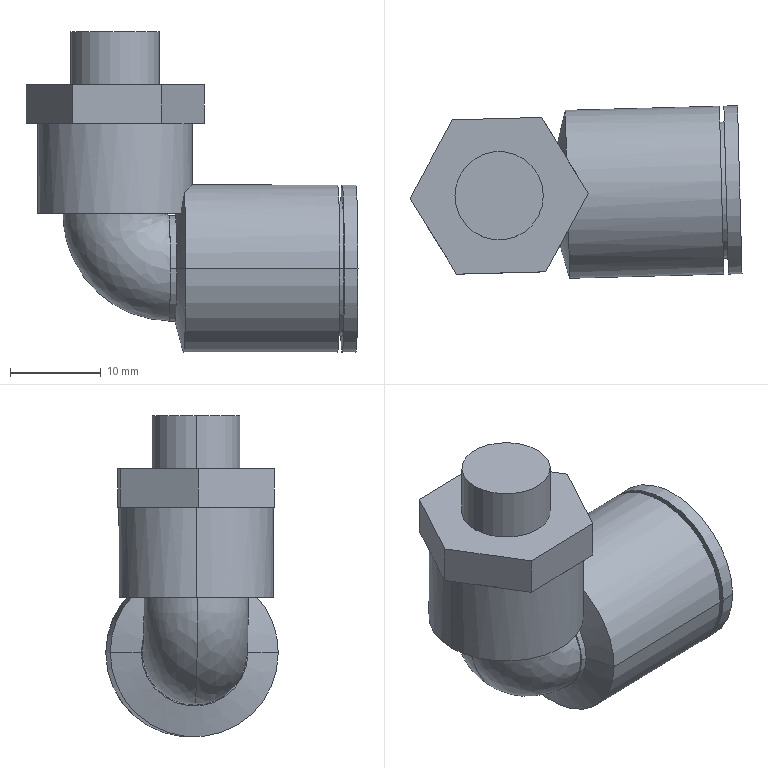Part | SolidWorks | features BaseBody 1 | 1 solid | 38 faces | box 36.549 x 18.999 x 35.35 mm | volume 8339 mm3 | plane 20 | cylinder 14 | cone 2 | spline 2 | commonest cylinder face diameters 18.5 x4 9.728 x2 10 x2 11.729 x2 15 x2 17 x2
STEP:
#1=CARTESIAN_POINT('',(84.738,-8.593,311.618));
#2=VERTEX_POINT('',#1);
#3=CARTESIAN_POINT('',(84.245,9.9,311.618));
#4=VERTEX_POINT('',#3);
#5=CARTESIAN_POINT('',(84.491,0.6533,311.618));
#6=DIRECTION('',(-0.9996,-0.02667,0.));
#7=DIRECTION('',(0.02667,-0.9996,0.));
#8=AXIS2_PLACEMENT_3D('',#5,#6,#7);
#9=CIRCLE('',#8,9.25);
#10=EDGE_CURVE('',#2,#4,#9,.T.);
#11=ORIENTED_EDGE('',*,*,#10,.T.);
#12=CARTESIAN_POINT('',(67.283,9.448,311.618));
#13=VERTEX_POINT('',#12);
#14=CARTESIAN_POINT('',(75.764,9.674,311.618));
#15=DIRECTION('',(-0.9996,-0.02667,0.));
#16=VECTOR('',#15,1000.);
#17=LINE('',#14,#16);
#18=EDGE_CURVE('',#4,#13,#17,.T.);
#19=ORIENTED_EDGE('',*,*,#18,.T.);
#20=CARTESIAN_POINT('',(67.424,4.139,319.987));
#21=VERTEX_POINT('',#20);
#22=CARTESIAN_POINT('',(67.529,0.2009,311.618));
#23=DIRECTION('',(0.9996,0.02667,0.));
#24=DIRECTION('',(0.02667,-0.9996,0.));
#25=AXIS2_PLACEMENT_3D('',#22,#23,#24);
#26=CIRCLE('',#25,9.25);
#27=EDGE_CURVE('',#13,#21,#26,.T.);
#28=ORIENTED_EDGE('',*,*,#27,.T.);
#29=CARTESIAN_POINT('',(68.5,0.,320.865));
#30=VERTEX_POINT('',#29);
#31=CARTESIAN_POINT('',(67.424,4.139,319.987));
#32=CARTESIAN_POINT('',(67.759,3.538,320.274));
#33=CARTESIAN_POINT('',(68.027,2.89,320.502));
#34=CARTESIAN_POINT('',(68.308,1.834,320.734));
#35=CARTESIAN_POINT('',(68.379,1.473,320.79));
#36=CARTESIAN_POINT('',(68.451,0.9265,320.843));
#37=CARTESIAN_POINT('',(68.47,0.7429,320.855));
#38=CARTESIAN_POINT('',(68.494,0.3729,320.869));
#39=CARTESIAN_POINT('',(68.5,0.1856,320.87));
#40=CARTESIAN_POINT('',(68.5,0.,320.865));
#41=B_SPLINE_CURVE_WITH_KNOTS('',3,(#31,#32,#33,#34,#35,#36,#37,#38,#39,#40),.UNSPECIFIED.,.F.,.F.,(4,2,2,2,4),(-0.004184,-0.00198,-0.0008783,-0.0003273,0.0002237),.UNSPECIFIED.);
#42=EDGE_CURVE('',#21,#30,#41,.T.);
#43=ORIENTED_EDGE('',*,*,#42,.T.);
#44=CARTESIAN_POINT('',(67.635,-3.737,319.987));
#45=VERTEX_POINT('',#44);
#46=CARTESIAN_POINT('',(68.5,0.,320.865));
#47=CARTESIAN_POINT('',(68.5,-0.6674,320.849));
#48=CARTESIAN_POINT('',(68.423,-1.318,320.761));
#49=CARTESIAN_POINT('',(68.198,-2.269,320.533));
#50=CARTESIAN_POINT('',(68.106,-2.577,320.442));
#51=CARTESIAN_POINT('',(67.892,-3.172,320.233));
#52=CARTESIAN_POINT('',(67.77,-3.459,320.116));
#53=CARTESIAN_POINT('',(67.635,-3.737,319.987));
#54=B_SPLINE_CURVE_WITH_KNOTS('',3,(#46,#47,#48,#49,#50,#51,#52,#53),.UNSPECIFIED.,.F.,.F.,(4,2,2,4),(0.0002237,0.002205,0.003196,0.004187),.UNSPECIFIED.);
#55=EDGE_CURVE('',#30,#45,#54,.T.);
#56=ORIENTED_EDGE('',*,*,#55,.T.);
#57=CARTESIAN_POINT('',(67.776,-9.046,311.618));
#58=VERTEX_POINT('',#57);
#59=CARTESIAN_POINT('',(67.529,0.2009,311.618));
#60=DIRECTION('',(0.9996,0.02667,0.));
#61=DIRECTION('',(0.02667,-0.9996,0.));
#62=AXIS2_PLACEMENT_3D('',#59,#60,#61);
#63=CIRCLE('',#62,9.25);
#64=EDGE_CURVE('',#45,#58,#63,.T.);
#65=ORIENTED_EDGE('',*,*,#64,.T.);
#66=CARTESIAN_POINT('',(76.257,-8.82,311.618));
#67=DIRECTION('',(-0.9996,-0.02667,0.));
#68=VECTOR('',#67,1000.);
#69=LINE('',#66,#68);
#70=EDGE_CURVE('',#2,#58,#69,.T.);
#71=ORIENTED_EDGE('',*,*,#70,.F.);
#72=EDGE_LOOP('',(#11,#19,#28,#43,#56,#65,#71));
#73=FACE_OUTER_BOUND('',#72,.T.);
#74=CARTESIAN_POINT('',(76.01,0.4271,311.618));
#75=DIRECTION('',(-0.9996,-0.02667,0.));
#76=DIRECTION('',(0.02667,-0.9996,0.));
#77=AXIS2_PLACEMENT_3D('',#74,#75,#76);
#78=CYLINDRICAL_SURFACE('',#77,9.25);
#79=ADVANCED_FACE('',(#73),#78,.T.);
#80=CARTESIAN_POINT('',(66.466,6.039,311.618));
#81=VERTEX_POINT('',#80);
#82=CARTESIAN_POINT('',(66.779,-5.686,311.618));
#83=VERTEX_POINT('',#82);
#84=CARTESIAN_POINT('',(66.623,0.1767,311.618));
#85=DIRECTION('',(0.9996,0.02667,0.));
#86=DIRECTION('',(-0.02667,0.9996,0.));
#87=AXIS2_PLACEMENT_3D('',#84,#85,#86);
#88=CIRCLE('',#87,5.864);
#89=EDGE_CURVE('',#81,#83,#88,.T.);
#90=ORIENTED_EDGE('',*,*,#89,.T.);
#91=CARTESIAN_POINT('',(67.776,-9.046,311.618));
#92=DIRECTION('',(0.2845,-0.9587,0.));
#93=VECTOR('',#92,1000.);
#94=LINE('',#91,#93);
#95=EDGE_CURVE('',#83,#58,#94,.T.);
#96=ORIENTED_EDGE('',*,*,#95,.T.);
#97=ORIENTED_EDGE('',*,*,#64,.F.);
#98=CARTESIAN_POINT('',(67.233,-4.465,317.723));
#99=VERTEX_POINT('',#98);
#100=CARTESIAN_POINT('',(67.635,-3.737,319.987));
#101=CARTESIAN_POINT('',(67.495,-4.022,319.247));
#102=CARTESIAN_POINT('',(67.358,-4.262,318.492));
#103=CARTESIAN_POINT('',(67.233,-4.465,317.723));
#104=B_SPLINE_CURVE_WITH_KNOTS('',3,(#100,#101,#102,#103),.UNSPECIFIED.,.F.,.F.,(4,4),(0.,0.002412),.UNSPECIFIED.);
#105=EDGE_CURVE('',#45,#99,#104,.T.);
#106=ORIENTED_EDGE('',*,*,#105,.T.);
#107=CARTESIAN_POINT('',(66.984,4.845,317.723));
#108=VERTEX_POINT('',#107);
#109=CARTESIAN_POINT('',(67.233,-4.465,317.723));
#110=CARTESIAN_POINT('',(67.087,-3.698,317.723));
#111=CARTESIAN_POINT('',(66.96,-2.928,317.723));
#112=CARTESIAN_POINT('',(66.77,-1.381,317.723));
#113=CARTESIAN_POINT('',(66.708,-0.6038,317.723));
#114=CARTESIAN_POINT('',(66.666,0.9606,317.723));
#115=CARTESIAN_POINT('',(66.687,1.74,317.723));
#116=CARTESIAN_POINT('',(66.794,3.295,317.723));
#117=CARTESIAN_POINT('',(66.88,4.07,317.723));
#118=CARTESIAN_POINT('',(66.984,4.845,317.723));
#119=B_SPLINE_CURVE_WITH_KNOTS('',3,(#109,#110,#111,#112,#113,#114,#115,#116,#117,#118),.UNSPECIFIED.,.F.,.F.,(4,2,2,2,4),(0.,0.002338,0.004676,0.007013,0.009351),.UNSPECIFIED.);
#120=EDGE_CURVE('',#99,#108,#119,.T.);
#121=ORIENTED_EDGE('',*,*,#120,.T.);
#122=CARTESIAN_POINT('',(67.424,4.139,319.987));
#123=CARTESIAN_POINT('',(67.27,4.416,319.247));
#124=CARTESIAN_POINT('',(67.121,4.648,318.492));
#125=CARTESIAN_POINT('',(66.984,4.845,317.723));
#126=B_SPLINE_CURVE_WITH_KNOTS('',3,(#122,#123,#124,#125),.UNSPECIFIED.,.F.,.F.,(4,4),(0.,0.002412),.UNSPECIFIED.);
#127=EDGE_CURVE('',#21,#108,#126,.T.);
#128=ORIENTED_EDGE('',*,*,#127,.F.);
#129=ORIENTED_EDGE('',*,*,#27,.F.);
#130=CARTESIAN_POINT('',(67.283,9.448,311.618));
#131=DIRECTION('',(0.233,0.9725,0.));
#132=VECTOR('',#131,1000.);
#133=LINE('',#130,#132);
#134=EDGE_CURVE('',#81,#13,#133,.T.);
#135=ORIENTED_EDGE('',*,*,#134,.F.);
#136=EDGE_LOOP('',(#90,#96,#97,#106,#121,#128,#129,#135));
#137=FACE_OUTER_BOUND('',#136,.T.);
#138=CARTESIAN_POINT('',(67.529,0.2009,311.618));
#139=DIRECTION('',(0.9996,0.02667,0.));
#140=DIRECTION('',(-0.02667,0.9996,0.));
#141=AXIS2_PLACEMENT_3D('',#138,#139,#140);
#142=CONICAL_SURFACE('',#141,9.25,1.309);
#143=ADVANCED_FACE('',(#137),#142,.T.);
#144=CARTESIAN_POINT('',(67.245,4.445,327.631));
#145=VERTEX_POINT('',#144);
#146=CARTESIAN_POINT('',(68.5,0.,327.631));
#147=VERTEX_POINT('',#146);
#148=CARTESIAN_POINT('',(60.,0.,327.631));
#149=DIRECTION('',(0.,0.,-1.));
#150=DIRECTION('',(-1.,0.,0.));
#151=AXIS2_PLACEMENT_3D('',#148,#149,#150);
#152=CIRCLE('',#151,8.5);
#153=EDGE_CURVE('',#145,#147,#152,.T.);
#154=ORIENTED_EDGE('',*,*,#153,.T.);
#155=CARTESIAN_POINT('',(68.5,0.,324.705));
#156=DIRECTION('',(0.,0.,-1.));
#157=VECTOR('',#156,1000.);
#158=LINE('',#155,#157);
#159=EDGE_CURVE('',#147,#30,#158,.T.);
#160=ORIENTED_EDGE('',*,*,#159,.T.);
#161=ORIENTED_EDGE('',*,*,#42,.F.);
#162=ORIENTED_EDGE('',*,*,#127,.T.);
#163=CARTESIAN_POINT('',(51.5,0.,317.723));
#164=VERTEX_POINT('',#163);
#165=CARTESIAN_POINT('',(60.,0.,317.723));
#166=DIRECTION('',(0.,0.,1.));
#167=DIRECTION('',(-1.,0.,0.));
#168=AXIS2_PLACEMENT_3D('',#165,#166,#167);
#169=CIRCLE('',#168,8.5);
#170=EDGE_CURVE('',#108,#164,#169,.T.);
#171=ORIENTED_EDGE('',*,*,#170,.T.);
#172=CARTESIAN_POINT('',(51.5,0.,327.631));
#173=VERTEX_POINT('',#172);
#174=CARTESIAN_POINT('',(51.5,0.,324.705));
#175=DIRECTION('',(0.,0.,-1.));
#176=VECTOR('',#175,1000.);
#177=LINE('',#174,#176);
#178=EDGE_CURVE('',#173,#164,#177,.T.);
#179=ORIENTED_EDGE('',*,*,#178,.F.);
#180=CARTESIAN_POINT('',(52.528,4.052,327.631));
#181=VERTEX_POINT('',#180);
#182=CARTESIAN_POINT('',(60.,0.,327.631));
#183=DIRECTION('',(0.,0.,-1.));
#184=DIRECTION('',(-1.,0.,0.));
#185=AXIS2_PLACEMENT_3D('',#182,#183,#184);
#186=CIRCLE('',#185,8.5);
#187=EDGE_CURVE('',#173,#181,#186,.T.);
#188=ORIENTED_EDGE('',*,*,#187,.T.);
#189=CARTESIAN_POINT('',(59.773,8.497,327.631));
#190=VERTEX_POINT('',#189);
#191=CARTESIAN_POINT('',(60.,0.,327.631));
#192=DIRECTION('',(0.,0.,-1.));
#193=DIRECTION('',(-1.,0.,0.));
#194=AXIS2_PLACEMENT_3D('',#191,#192,#193);
#195=CIRCLE('',#194,8.5);
#196=EDGE_CURVE('',#181,#190,#195,.T.);
#197=ORIENTED_EDGE('',*,*,#196,.T.);
#198=CARTESIAN_POINT('',(60.,0.,327.631));
#199=DIRECTION('',(0.,0.,-1.));
#200=DIRECTION('',(-1.,0.,0.));
#201=AXIS2_PLACEMENT_3D('',#198,#199,#200);
#202=CIRCLE('',#201,8.5);
#203=EDGE_CURVE('',#190,#145,#202,.T.);
#204=ORIENTED_EDGE('',*,*,#203,.T.);
#205=EDGE_LOOP('',(#154,#160,#161,#162,#171,#179,#188,#197,#204));
#206=FACE_OUTER_BOUND('',#205,.T.);
#207=CARTESIAN_POINT('',(60.,0.,324.705));
#208=DIRECTION('',(0.,0.,-1.));
#209=DIRECTION('',(-1.,0.,0.));
#210=AXIS2_PLACEMENT_3D('',#207,#208,#209);
#211=CYLINDRICAL_SURFACE('',#210,8.5);
#212=ADVANCED_FACE('',(#206),#211,.T.);
#213=ORIENTED_EDGE('',*,*,#89,.F.);
#214=CARTESIAN_POINT('',(65.762,6.02,311.618));
#215=VERTEX_POINT('',#214);
#216=CARTESIAN_POINT('',(66.114,6.03,311.618));
#217=DIRECTION('',(-0.9996,-0.02667,0.));
#218=VECTOR('',#217,1000.);
#219=LINE('',#216,#218);
#220=EDGE_CURVE('',#81,#215,#219,.T.);
#221=ORIENTED_EDGE('',*,*,#220,.T.);
#222=CARTESIAN_POINT('',(66.074,-5.705,311.618));
#223=VERTEX_POINT('',#222);
#224=CARTESIAN_POINT('',(65.918,0.1579,311.618));
#225=DIRECTION('',(0.9996,0.02667,0.));
#226=DIRECTION('',(0.02667,-0.9996,0.));
#227=AXIS2_PLACEMENT_3D('',#224,#225,#226);
#228=CIRCLE('',#227,5.865);
#229=EDGE_CURVE('',#215,#223,#228,.T.);
#230=ORIENTED_EDGE('',*,*,#229,.T.);
#231=CARTESIAN_POINT('',(66.427,-5.695,311.618));
#232=DIRECTION('',(-0.9996,-0.02667,0.));
#233=VECTOR('',#232,1000.);
#234=LINE('',#231,#233);
#235=EDGE_CURVE('',#83,#223,#234,.T.);
#236=ORIENTED_EDGE('',*,*,#235,.F.);
#237=EDGE_LOOP('',(#213,#221,#230,#236));
#238=FACE_OUTER_BOUND('',#237,.T.);
#239=CARTESIAN_POINT('',(66.27,0.1673,311.618));
#240=DIRECTION('',(-0.9996,-0.02667,0.));
#241=DIRECTION('',(0.02667,-0.9996,0.));
#242=AXIS2_PLACEMENT_3D('',#239,#240,#241);
#243=CYLINDRICAL_SURFACE('',#242,5.865);
#244=ADVANCED_FACE('',(#238),#243,.T.);
#245=CARTESIAN_POINT('',(85.191,-6.831,311.618));
#246=VERTEX_POINT('',#245);
#247=CARTESIAN_POINT('',(84.791,8.164,311.618));
#248=VERTEX_POINT('',#247);
#249=CARTESIAN_POINT('',(84.991,0.6666,311.618));
#250=DIRECTION('',(-0.9996,-0.02667,0.));
#251=DIRECTION('',(0.02667,-0.9996,0.));
#252=AXIS2_PLACEMENT_3D('',#249,#250,#251);
#253=CIRCLE('',#252,7.5);
#254=EDGE_CURVE('',#246,#248,#253,.T.);
#255=ORIENTED_EDGE('',*,*,#254,.T.);
#256=CARTESIAN_POINT('',(84.291,8.151,311.618));
#257=VERTEX_POINT('',#256);
#258=CARTESIAN_POINT('',(84.541,8.157,311.618));
#259=DIRECTION('',(-0.9996,-0.02667,0.));
#260=VECTOR('',#259,1000.);
#261=LINE('',#258,#260);
#262=EDGE_CURVE('',#248,#257,#261,.T.);
#263=ORIENTED_EDGE('',*,*,#262,.T.);
#264=CARTESIAN_POINT('',(84.691,-6.844,311.618));
#265=VERTEX_POINT('',#264);
#266=CARTESIAN_POINT('',(84.491,0.6533,311.618));
#267=DIRECTION('',(-0.9996,-0.02667,0.));
#268=DIRECTION('',(0.02667,-0.9996,0.));
#269=AXIS2_PLACEMENT_3D('',#266,#267,#268);
#270=CIRCLE('',#269,7.5);
#271=EDGE_CURVE('',#265,#257,#270,.T.);
#272=ORIENTED_EDGE('',*,*,#271,.F.);
#273=CARTESIAN_POINT('',(84.941,-6.837,311.618));
#274=DIRECTION('',(-0.9996,-0.02667,0.));
#275=VECTOR('',#274,1000.);
#276=LINE('',#273,#275);
#277=EDGE_CURVE('',#246,#265,#276,.T.);
#278=ORIENTED_EDGE('',*,*,#277,.F.);
#279=EDGE_LOOP('',(#255,#263,#272,#278));
#280=FACE_OUTER_BOUND('',#279,.T.);
#281=CARTESIAN_POINT('',(84.741,0.66,311.618));
#282=DIRECTION('',(-0.9996,-0.02667,0.));
#283=DIRECTION('',(0.02667,-0.9996,0.));
#284=AXIS2_PLACEMENT_3D('',#281,#282,#283);
#285=CYLINDRICAL_SURFACE('',#284,7.5);
#286=ADVANCED_FACE('',(#280),#285,.T.);
#287=CARTESIAN_POINT('',(86.737,-8.54,311.618));
#288=VERTEX_POINT('',#287);
#289=CARTESIAN_POINT('',(86.244,9.953,311.618));
#290=VERTEX_POINT('',#289);
#291=CARTESIAN_POINT('',(86.491,0.7066,311.618));
#292=DIRECTION('',(-0.9996,-0.02667,0.));
#293=DIRECTION('',(0.02667,-0.9996,0.));
#294=AXIS2_PLACEMENT_3D('',#291,#292,#293);
#295=CIRCLE('',#294,9.25);
#296=EDGE_CURVE('',#288,#290,#295,.T.);
#297=ORIENTED_EDGE('',*,*,#296,.T.);
#298=CARTESIAN_POINT('',(84.744,9.913,311.618));
#299=VERTEX_POINT('',#298);
#300=CARTESIAN_POINT('',(85.494,9.933,311.618));
#301=DIRECTION('',(-0.9996,-0.02667,0.));
#302=VECTOR('',#301,1000.);
#303=LINE('',#300,#302);
#304=EDGE_CURVE('',#290,#299,#303,.T.);
#305=ORIENTED_EDGE('',*,*,#304,.T.);
#306=CARTESIAN_POINT('',(85.238,-8.58,311.618));
#307=VERTEX_POINT('',#306);
#308=CARTESIAN_POINT('',(84.991,0.6666,311.618));
#309=DIRECTION('',(-0.9996,-0.02667,0.));
#310=DIRECTION('',(0.02667,-0.9996,0.));
#311=AXIS2_PLACEMENT_3D('',#308,#309,#310);
#312=CIRCLE('',#311,9.25);
#313=EDGE_CURVE('',#307,#299,#312,.T.);
#314=ORIENTED_EDGE('',*,*,#313,.F.);
#315=CARTESIAN_POINT('',(85.988,-8.56,311.618));
#316=DIRECTION('',(-0.9996,-0.02667,0.));
#317=VECTOR('',#316,1000.);
#318=LINE('',#315,#317);
#319=EDGE_CURVE('',#288,#307,#318,.T.);
#320=ORIENTED_EDGE('',*,*,#319,.F.);
#321=EDGE_LOOP('',(#297,#305,#314,#320));
#322=FACE_OUTER_BOUND('',#321,.T.);
#323=CARTESIAN_POINT('',(85.741,0.6866,311.618));
#324=DIRECTION('',(-0.9996,-0.02667,0.));
#325=DIRECTION('',(0.02667,-0.9996,0.));
#326=AXIS2_PLACEMENT_3D('',#323,#324,#325);
#327=CYLINDRICAL_SURFACE('',#326,9.25);
#328=ADVANCED_FACE('',(#322),#327,.T.);
#329=CARTESIAN_POINT('',(55.136,0.,337.718));
#330=VERTEX_POINT('',#329);
#331=CARTESIAN_POINT('',(64.864,0.,337.718));
#332=VERTEX_POINT('',#331);
#333=CARTESIAN_POINT('',(60.,0.,337.718));
#334=DIRECTION('',(0.,0.,-1.));
#335=DIRECTION('',(-1.,0.,0.));
#336=AXIS2_PLACEMENT_3D('',#333,#334,#335);
#337=CIRCLE('',#336,4.864);
#338=EDGE_CURVE('',#330,#332,#337,.T.);
#339=ORIENTED_EDGE('',*,*,#338,.T.);
#340=CARTESIAN_POINT('',(64.864,0.,331.881));
#341=VERTEX_POINT('',#340);
#342=CARTESIAN_POINT('',(64.864,0.,334.702));
#343=DIRECTION('',(0.,0.,-1.));
#344=VECTOR('',#343,1000.);
#345=LINE('',#342,#344);
#346=EDGE_CURVE('',#332,#341,#345,.T.);
#347=ORIENTED_EDGE('',*,*,#346,.T.);
#348=CARTESIAN_POINT('',(55.136,0.,331.881));
#349=VERTEX_POINT('',#348);
#350=CARTESIAN_POINT('',(60.,0.,331.881));
#351=DIRECTION('',(0.,0.,1.));
#352=DIRECTION('',(-1.,0.,0.));
#353=AXIS2_PLACEMENT_3D('',#350,#351,#352);
#354=CIRCLE('',#353,4.864);
#355=EDGE_CURVE('',#341,#349,#354,.T.);
#356=ORIENTED_EDGE('',*,*,#355,.T.);
#357=CARTESIAN_POINT('',(55.136,0.,334.702));
#358=DIRECTION('',(0.,0.,-1.));
#359=VECTOR('',#358,1000.);
#360=LINE('',#357,#359);
#361=EDGE_CURVE('',#330,#349,#360,.T.);
#362=ORIENTED_EDGE('',*,*,#361,.F.);
#363=EDGE_LOOP('',(#339,#347,#356,#362));
#364=FACE_OUTER_BOUND('',#363,.T.);
#365=CARTESIAN_POINT('',(60.,0.,334.702));
#366=DIRECTION('',(0.,0.,-1.));
#367=DIRECTION('',(-1.,0.,0.));
#368=AXIS2_PLACEMENT_3D('',#365,#366,#367);
#369=CYLINDRICAL_SURFACE('',#368,4.864);
#370=ADVANCED_FACE('',(#364),#369,.T.);
#371=CARTESIAN_POINT('',(65.631,-4.852,311.618));
#372=VERTEX_POINT('',#371);
#373=CARTESIAN_POINT('',(65.365,5.145,311.618));
#374=VERTEX_POINT('',#373);
#375=CARTESIAN_POINT('',(65.498,0.1467,311.618));
#376=DIRECTION('',(0.9996,0.02667,0.));
#377=DIRECTION('',(-0.02667,0.9996,0.));
#378=AXIS2_PLACEMENT_3D('',#375,#376,#377);
#379=CIRCLE('',#378,5.);
#380=EDGE_CURVE('',#372,#374,#379,.T.);
#381=ORIENTED_EDGE('',*,*,#380,.F.);
#382=CARTESIAN_POINT('',(86.624,-4.292,311.618));
#383=VERTEX_POINT('',#382);
#384=CARTESIAN_POINT('',(107.616,-3.732,311.618));
#385=DIRECTION('',(0.9996,0.02667,0.));
#386=VECTOR('',#385,1000.);
#387=LINE('',#384,#386);
#388=EDGE_CURVE('',#372,#383,#387,.T.);
#389=ORIENTED_EDGE('',*,*,#388,.T.);
#390=CARTESIAN_POINT('',(86.357,5.705,311.618));
#391=VERTEX_POINT('',#390);
#392=CARTESIAN_POINT('',(86.491,0.7066,311.618));
#393=DIRECTION('',(-0.9996,-0.02667,0.));
#394=DIRECTION('',(-0.02667,0.9996,0.));
#395=AXIS2_PLACEMENT_3D('',#392,#393,#394);
#396=CIRCLE('',#395,5.);
#397=EDGE_CURVE('',#391,#383,#396,.T.);
#398=ORIENTED_EDGE('',*,*,#397,.F.);
#399=CARTESIAN_POINT('',(107.35,6.265,311.618));
#400=DIRECTION('',(0.9996,0.02667,0.));
#401=VECTOR('',#400,1000.);
#402=LINE('',#399,#401);
#403=EDGE_CURVE('',#374,#391,#402,.T.);
#404=ORIENTED_EDGE('',*,*,#403,.F.);
#405=EDGE_LOOP('',(#381,#389,#398,#404));
#406=FACE_OUTER_BOUND('',#405,.T.);
#407=CARTESIAN_POINT('',(107.483,1.267,311.618));
#408=DIRECTION('',(0.9996,0.02667,0.));
#409=DIRECTION('',(-0.02667,0.9996,0.));
#410=AXIS2_PLACEMENT_3D('',#407,#408,#409);
#411=CYLINDRICAL_SURFACE('',#410,5.);
#412=ADVANCED_FACE('',(#406),#411,.F.);
#413=ORIENTED_EDGE('',*,*,#18,.F.);
#414=CARTESIAN_POINT('',(84.491,0.6533,311.618));
#415=DIRECTION('',(-0.9996,-0.02667,0.));
#416=DIRECTION('',(0.02667,-0.9996,0.));
#417=AXIS2_PLACEMENT_3D('',#414,#415,#416);
#418=CIRCLE('',#417,9.25);
#419=EDGE_CURVE('',#4,#2,#418,.T.);
#420=ORIENTED_EDGE('',*,*,#419,.T.);
#421=ORIENTED_EDGE('',*,*,#70,.T.);
#422=CARTESIAN_POINT('',(67.529,0.2009,311.618));
#423=DIRECTION('',(0.9996,0.02667,0.));
#424=DIRECTION('',(0.02667,-0.9996,0.));
#425=AXIS2_PLACEMENT_3D('',#422,#423,#424);
#426=CIRCLE('',#425,9.25);
#427=EDGE_CURVE('',#58,#13,#426,.T.);
#428=ORIENTED_EDGE('',*,*,#427,.T.);
#429=EDGE_LOOP('',(#413,#420,#421,#428));
#430=FACE_OUTER_BOUND('',#429,.T.);
#431=CARTESIAN_POINT('',(76.01,0.4271,311.618));
#432=DIRECTION('',(-0.9996,-0.02667,0.));
#433=DIRECTION('',(0.02667,-0.9996,0.));
#434=AXIS2_PLACEMENT_3D('',#431,#432,#433);
#435=CYLINDRICAL_SURFACE('',#434,9.25);
#436=ADVANCED_FACE('',(#430),#435,.T.);
#437=ORIENTED_EDGE('',*,*,#95,.F.);
#438=CARTESIAN_POINT('',(66.623,0.1767,311.618));
#439=DIRECTION('',(0.9996,0.02667,0.));
#440=DIRECTION('',(-0.02667,0.9996,0.));
#441=AXIS2_PLACEMENT_3D('',#438,#439,#440);
#442=CIRCLE('',#441,5.864);
#443=EDGE_CURVE('',#83,#81,#442,.T.);
#444=ORIENTED_EDGE('',*,*,#443,.T.);
#445=ORIENTED_EDGE('',*,*,#134,.T.);
#446=ORIENTED_EDGE('',*,*,#427,.F.);
#447=EDGE_LOOP('',(#437,#444,#445,#446));
#448=FACE_OUTER_BOUND('',#447,.T.);
#449=CARTESIAN_POINT('',(67.529,0.2009,311.618));
#450=DIRECTION('',(0.9996,0.02667,0.));
#451=DIRECTION('',(-0.02667,0.9996,0.));
#452=AXIS2_PLACEMENT_3D('',#449,#450,#451);
#453=CONICAL_SURFACE('',#452,9.25,1.309);
#454=ADVANCED_FACE('',(#448),#453,.T.);
#455=ORIENTED_EDGE('',*,*,#159,.F.);
#456=CARTESIAN_POINT('',(67.472,-4.052,327.631));
#457=VERTEX_POINT('',#456);
#458=CARTESIAN_POINT('',(60.,0.,327.631));
#459=DIRECTION('',(0.,0.,-1.));
#460=DIRECTION('',(-1.,0.,0.));
#461=AXIS2_PLACEMENT_3D('',#458,#459,#460);
#462=CIRCLE('',#461,8.5);
#463=EDGE_CURVE('',#147,#457,#462,.T.);
#464=ORIENTED_EDGE('',*,*,#463,.T.);
#465=CARTESIAN_POINT('',(60.227,-8.497,327.631));
#466=VERTEX_POINT('',#465);
#467=CARTESIAN_POINT('',(60.,0.,327.631));
#468=DIRECTION('',(0.,0.,-1.));
#469=DIRECTION('',(-1.,0.,0.));
#470=AXIS2_PLACEMENT_3D('',#467,#468,#469);
#471=CIRCLE('',#470,8.5);
#472=EDGE_CURVE('',#457,#466,#471,.T.);
#473=ORIENTED_EDGE('',*,*,#472,.T.);
#474=CARTESIAN_POINT('',(52.755,-4.445,327.631));
#475=VERTEX_POINT('',#474);
#476=CARTESIAN_POINT('',(60.,0.,327.631));
#477=DIRECTION('',(0.,0.,-1.));
#478=DIRECTION('',(-1.,0.,0.));
#479=AXIS2_PLACEMENT_3D('',#476,#477,#478);
#480=CIRCLE('',#479,8.5);
#481=EDGE_CURVE('',#466,#475,#480,.T.);
#482=ORIENTED_EDGE('',*,*,#481,.T.);
#483=CARTESIAN_POINT('',(60.,0.,327.631));
#484=DIRECTION('',(0.,0.,-1.));
#485=DIRECTION('',(-1.,0.,0.));
#486=AXIS2_PLACEMENT_3D('',#483,#484,#485);
#487=CIRCLE('',#486,8.5);
#488=EDGE_CURVE('',#475,#173,#487,.T.);
#489=ORIENTED_EDGE('',*,*,#488,.T.);
#490=ORIENTED_EDGE('',*,*,#178,.T.);
#491=CARTESIAN_POINT('',(60.,0.,317.723));
#492=DIRECTION('',(0.,0.,1.));
#493=DIRECTION('',(-1.,0.,0.));
#494=AXIS2_PLACEMENT_3D('',#491,#492,#493);
#495=CIRCLE('',#494,8.5);
#496=EDGE_CURVE('',#164,#99,#495,.T.);
#497=ORIENTED_EDGE('',*,*,#496,.T.);
#498=ORIENTED_EDGE('',*,*,#105,.F.);
#499=ORIENTED_EDGE('',*,*,#55,.F.);
#500=EDGE_LOOP('',(#455,#464,#473,#482,#489,#490,#497,#498,#499));
#501=FACE_OUTER_BOUND('',#500,.T.);
#502=CARTESIAN_POINT('',(60.,0.,324.705));
#503=DIRECTION('',(0.,0.,-1.));
#504=DIRECTION('',(-1.,0.,0.));
#505=AXIS2_PLACEMENT_3D('',#502,#503,#504);
#506=CYLINDRICAL_SURFACE('',#505,8.5);
#507=ADVANCED_FACE('',(#501),#506,.T.);
#508=ORIENTED_EDGE('',*,*,#271,.T.);
#509=CARTESIAN_POINT('',(84.491,0.6533,311.618));
#510=DIRECTION('',(-0.9996,-0.02667,0.));
#511=DIRECTION('',(0.02667,-0.9996,0.));
#512=AXIS2_PLACEMENT_3D('',#509,#510,#511);
#513=CIRCLE('',#512,7.5);
#514=EDGE_CURVE('',#257,#265,#513,.T.);
#515=ORIENTED_EDGE('',*,*,#514,.T.);
#516=EDGE_LOOP('',(#508,#515));
#517=FACE_BOUND('',#516,.T.);
#518=ORIENTED_EDGE('',*,*,#10,.F.);
#519=ORIENTED_EDGE('',*,*,#419,.F.);
#520=EDGE_LOOP('',(#518,#519));
#521=FACE_OUTER_BOUND('',#520,.T.);
#522=CARTESIAN_POINT('',(84.268,9.025,311.618));
#523=DIRECTION('',(0.9996,0.02667,0.));
#524=DIRECTION('',(-0.02667,0.9996,0.));
#525=AXIS2_PLACEMENT_3D('',#522,#523,#524);
#526=PLANE('',#525);
#527=ADVANCED_FACE('',(#517,#521),#526,.T.);
#528=ORIENTED_EDGE('',*,*,#220,.F.);
#529=ORIENTED_EDGE('',*,*,#443,.F.);
#530=ORIENTED_EDGE('',*,*,#235,.T.);
#531=CARTESIAN_POINT('',(65.918,0.1579,311.618));
#532=DIRECTION('',(0.9996,0.02667,0.));
#533=DIRECTION('',(0.02667,-0.9996,0.));
#534=AXIS2_PLACEMENT_3D('',#531,#532,#533);
#535=CIRCLE('',#534,5.865);
#536=EDGE_CURVE('',#223,#215,#535,.T.);
#537=ORIENTED_EDGE('',*,*,#536,.T.);
#538=EDGE_LOOP('',(#528,#529,#530,#537));
#539=FACE_OUTER_BOUND('',#538,.T.);
#540=CARTESIAN_POINT('',(66.27,0.1673,311.618));
#541=DIRECTION('',(-0.9996,-0.02667,0.));
#542=DIRECTION('',(0.02667,-0.9996,0.));
#543=AXIS2_PLACEMENT_3D('',#540,#541,#542);
#544=CYLINDRICAL_SURFACE('',#543,5.865);
#545=ADVANCED_FACE('',(#539),#544,.T.);
#546=ORIENTED_EDGE('',*,*,#120,.F.);
#547=ORIENTED_EDGE('',*,*,#496,.F.);
#548=ORIENTED_EDGE('',*,*,#170,.F.);
#549=EDGE_LOOP('',(#546,#547,#548));
#550=FACE_OUTER_BOUND('',#549,.T.);
#551=CARTESIAN_POINT('',(54.267,-0.1529,317.723));
#552=VERTEX_POINT('',#551);
#553=CARTESIAN_POINT('',(65.733,0.1529,317.723));
#554=VERTEX_POINT('',#553);
#555=CARTESIAN_POINT('',(54.267,-0.1529,317.723));
#556=CARTESIAN_POINT('',(54.573,-11.619,317.723));
#557=CARTESIAN_POINT('',(66.039,-11.313,317.723));
#558=CARTESIAN_POINT('',(65.733,0.1529,317.723));
#559=(BOUNDED_CURVE()B_SPLINE_CURVE(3,(#555,#556,#557,#558),.UNSPECIFIED.,.F.,.F.)B_SPLINE_CURVE_WITH_KNOTS((4,4),(0.,0.01793),.UNSPECIFIED.)CURVE()GEOMETRIC_REPRESENTATION_ITEM()RATIONAL_B_SPLINE_CURVE((1.,0.3333,0.3333,1.))REPRESENTATION_ITEM(''));
#560=EDGE_CURVE('',#552,#554,#559,.T.);
#561=ORIENTED_EDGE('',*,*,#560,.T.);
#562=CARTESIAN_POINT('',(65.733,0.1529,317.723));
#563=CARTESIAN_POINT('',(65.427,11.619,317.723));
#564=CARTESIAN_POINT('',(53.961,11.313,317.723));
#565=CARTESIAN_POINT('',(54.267,-0.1529,317.723));
#566=(BOUNDED_CURVE()B_SPLINE_CURVE(3,(#562,#563,#564,#565),.UNSPECIFIED.,.F.,.F.)B_SPLINE_CURVE_WITH_KNOTS((4,4),(0.,0.01814),.UNSPECIFIED.)CURVE()GEOMETRIC_REPRESENTATION_ITEM()RATIONAL_B_SPLINE_CURVE((1.,0.3333,0.3333,1.))REPRESENTATION_ITEM(''));
#567=EDGE_CURVE('',#554,#552,#566,.T.);
#568=ORIENTED_EDGE('',*,*,#567,.T.);
#569=EDGE_LOOP('',(#561,#568));
#570=FACE_BOUND('',#569,.T.);
#571=CARTESIAN_POINT('',(59.887,4.248,317.723));
#572=DIRECTION('',(0.,0.,-1.));
#573=DIRECTION('',(-1.,0.,0.));
#574=AXIS2_PLACEMENT_3D('',#571,#572,#573);
#575=PLANE('',#574);
#576=ADVANCED_FACE('',(#550,#570),#575,.T.);
#577=CARTESIAN_POINT('',(65.132,-8.366,327.631));
#578=VERTEX_POINT('',#577);
#579=CARTESIAN_POINT('',(65.132,-8.366,327.631));
#580=DIRECTION('',(-0.9996,-0.02667,0.));
#581=VECTOR('',#580,1000.);
#582=LINE('',#579,#581);
#583=EDGE_CURVE('',#578,#466,#582,.T.);
#584=ORIENTED_EDGE('',*,*,#583,.T.);
#585=ORIENTED_EDGE('',*,*,#472,.F.);
#586=CARTESIAN_POINT('',(67.472,-4.052,327.631));
#587=DIRECTION('',(-0.4767,-0.8791,0.));
#588=VECTOR('',#587,1000.);
#589=LINE('',#586,#588);
#590=EDGE_CURVE('',#457,#578,#589,.T.);
#591=ORIENTED_EDGE('',*,*,#590,.T.);
#592=EDGE_LOOP('',(#584,#585,#591));
#593=FACE_OUTER_BOUND('',#592,.T.);
#594=CARTESIAN_POINT('',(60.,0.,327.631));
#595=DIRECTION('',(0.,0.,-1.));
#596=DIRECTION('',(-1.,0.,0.));
#597=AXIS2_PLACEMENT_3D('',#594,#595,#596);
#598=PLANE('',#597);
#599=ADVANCED_FACE('',(#593),#598,.T.);
#600=CARTESIAN_POINT('',(69.811,0.2617,327.631));
#601=VERTEX_POINT('',#600);
#602=CARTESIAN_POINT('',(69.811,0.2617,327.631));
#603=DIRECTION('',(-0.4767,-0.8791,0.));
#604=VECTOR('',#603,1000.);
#605=LINE('',#602,#604);
#606=EDGE_CURVE('',#601,#457,#605,.T.);
#607=ORIENTED_EDGE('',*,*,#606,.T.);
#608=ORIENTED_EDGE('',*,*,#463,.F.);
#609=ORIENTED_EDGE('',*,*,#153,.F.);
#610=CARTESIAN_POINT('',(67.245,4.445,327.631));
#611=DIRECTION('',(0.5229,-0.8524,0.));
#612=VECTOR('',#611,1000.);
#613=LINE('',#610,#612);
#614=EDGE_CURVE('',#145,#601,#613,.T.);
#615=ORIENTED_EDGE('',*,*,#614,.T.);
#616=EDGE_LOOP('',(#607,#608,#609,#615));
#617=FACE_OUTER_BOUND('',#616,.T.);
#618=CARTESIAN_POINT('',(60.,0.,327.631));
#619=DIRECTION('',(0.,0.,-1.));
#620=DIRECTION('',(-1.,0.,0.));
#621=AXIS2_PLACEMENT_3D('',#618,#619,#620);
#622=PLANE('',#621);
#623=ADVANCED_FACE('',(#617),#622,.T.);
#624=CARTESIAN_POINT('',(64.679,8.628,327.631));
#625=VERTEX_POINT('',#624);
#626=CARTESIAN_POINT('',(64.679,8.628,327.631));
#627=DIRECTION('',(0.5229,-0.8524,0.));
#628=VECTOR('',#627,1000.);
#629=LINE('',#626,#628);
#630=EDGE_CURVE('',#625,#145,#629,.T.);
#631=ORIENTED_EDGE('',*,*,#630,.T.);
#632=ORIENTED_EDGE('',*,*,#203,.F.);
#633=CARTESIAN_POINT('',(59.773,8.497,327.631));
#634=DIRECTION('',(0.9996,0.02667,0.));
#635=VECTOR('',#634,1000.);
#636=LINE('',#633,#635);
#637=EDGE_CURVE('',#190,#625,#636,.T.);
#638=ORIENTED_EDGE('',*,*,#637,.T.);
#639=EDGE_LOOP('',(#631,#632,#638));
#640=FACE_OUTER_BOUND('',#639,.T.);
#641=CARTESIAN_POINT('',(60.,0.,327.631));
#642=DIRECTION('',(0.,0.,-1.));
#643=DIRECTION('',(-1.,0.,0.));
#644=AXIS2_PLACEMENT_3D('',#641,#642,#643);
#645=PLANE('',#644);
#646=ADVANCED_FACE('',(#640),#645,.T.);
#647=ORIENTED_EDGE('',*,*,#262,.F.);
#648=CARTESIAN_POINT('',(84.991,0.6666,311.618));
#649=DIRECTION('',(-0.9996,-0.02667,0.));
#650=DIRECTION('',(0.02667,-0.9996,0.));
#651=AXIS2_PLACEMENT_3D('',#648,#649,#650);
#652=CIRCLE('',#651,7.5);
#653=EDGE_CURVE('',#248,#246,#652,.T.);
#654=ORIENTED_EDGE('',*,*,#653,.T.);
#655=ORIENTED_EDGE('',*,*,#277,.T.);
#656=ORIENTED_EDGE('',*,*,#514,.F.);
#657=EDGE_LOOP('',(#647,#654,#655,#656));
#658=FACE_OUTER_BOUND('',#657,.T.);
#659=CARTESIAN_POINT('',(84.741,0.66,311.618));
#660=DIRECTION('',(-0.9996,-0.02667,0.));
#661=DIRECTION('',(0.02667,-0.9996,0.));
#662=AXIS2_PLACEMENT_3D('',#659,#660,#661);
#663=CYLINDRICAL_SURFACE('',#662,7.5);
#664=ADVANCED_FACE('',(#658),#663,.T.);
#665=ORIENTED_EDGE('',*,*,#536,.F.);
#666=ORIENTED_EDGE('',*,*,#229,.F.);
#667=EDGE_LOOP('',(#665,#666));
#668=FACE_OUTER_BOUND('',#667,.T.);
#669=CARTESIAN_POINT('',(65.918,0.1579,305.884));
#670=VERTEX_POINT('',#669);
#671=CARTESIAN_POINT('',(65.918,0.1579,317.402));
#672=VERTEX_POINT('',#671);
#673=CARTESIAN_POINT('',(65.918,0.1579,305.884));
#674=CARTESIAN_POINT('',(65.908,0.5369,305.884));
#675=CARTESIAN_POINT('',(65.898,0.9164,305.922));
#676=CARTESIAN_POINT('',(65.878,1.653,306.07));
#677=CARTESIAN_POINT('',(65.868,2.01,306.179));
#678=CARTESIAN_POINT('',(65.85,2.704,306.467));
#679=CARTESIAN_POINT('',(65.841,3.04,306.648));
#680=CARTESIAN_POINT('',(65.824,3.661,307.064));
#681=CARTESIAN_POINT('',(65.817,3.95,307.302));
#682=CARTESIAN_POINT('',(65.802,4.484,307.837));
#683=CARTESIAN_POINT('',(65.796,4.722,308.13));
#684=CARTESIAN_POINT('',(65.788,5.033,308.596));
#685=CARTESIAN_POINT('',(65.785,5.129,308.757));
#686=CARTESIAN_POINT('',(65.781,5.306,309.089));
#687=CARTESIAN_POINT('',(65.778,5.387,309.261));
#688=CARTESIAN_POINT('',(65.773,5.602,309.784));
#689=CARTESIAN_POINT('',(65.77,5.71,310.142));
#690=CARTESIAN_POINT('',(65.766,5.855,310.877));
#691=CARTESIAN_POINT('',(65.765,5.892,311.257));
#692=CARTESIAN_POINT('',(65.765,5.89,312.007));
#693=CARTESIAN_POINT('',(65.766,5.853,312.379));
#694=CARTESIAN_POINT('',(65.769,5.742,312.933));
#695=CARTESIAN_POINT('',(65.77,5.696,313.118));
#696=CARTESIAN_POINT('',(65.773,5.586,313.478));
#697=CARTESIAN_POINT('',(65.775,5.522,313.654));
#698=CARTESIAN_POINT('',(65.781,5.307,314.172));
#699=CARTESIAN_POINT('',(65.785,5.13,314.503));
#700=CARTESIAN_POINT('',(65.796,4.709,315.132));
#701=CARTESIAN_POINT('',(65.803,4.471,315.422));
#702=CARTESIAN_POINT('',(65.813,4.075,315.819));
#703=CARTESIAN_POINT('',(65.817,3.936,315.945));
#704=CARTESIAN_POINT('',(65.825,3.645,316.185));
#705=CARTESIAN_POINT('',(65.829,3.493,316.298));
#706=CARTESIAN_POINT('',(65.841,3.025,316.613));
#707=CARTESIAN_POINT('',(65.85,2.696,316.791));
#708=CARTESIAN_POINT('',(65.869,2.006,317.085));
#709=CARTESIAN_POINT('',(65.878,1.642,317.201));
#710=CARTESIAN_POINT('',(65.898,0.9097,317.359));
#711=CARTESIAN_POINT('',(65.908,0.5375,317.402));
#712=CARTESIAN_POINT('',(65.918,0.1579,317.402));
#713=B_SPLINE_CURVE_WITH_KNOTS('',3,(#673,#674,#675,#676,#677,#678,#679,#680,#681,#682,#683,#684,#685,#686,#687,#688,#689,#690,#691,#692,#693,#694,#695,#696,#697,#698,#699,#700,#701,#702,#703,#704,#705,#706,#707,#708,#709,#710,#711,#712),.UNSPECIFIED.,.F.,.F.,(4,2,2,2,2,2,2,2,2,2,2,2,2,2,2,2,2,2,2,4),(0.,0.001135,0.00227,0.003405,0.004541,0.005676,0.006243,0.006811,0.007946,0.009081,0.01022,0.01078,0.01135,0.01249,0.01362,0.01419,0.01476,0.01589,0.01703,0.01816),.UNSPECIFIED.);
#714=EDGE_CURVE('',#670,#672,#713,.T.);
#715=ORIENTED_EDGE('',*,*,#714,.T.);
#716=CARTESIAN_POINT('',(65.918,0.1579,317.402));
#717=CARTESIAN_POINT('',(65.928,-0.2213,317.402));
#718=CARTESIAN_POINT('',(65.938,-0.6003,317.358));
#719=CARTESIAN_POINT('',(65.958,-1.334,317.199));
#720=CARTESIAN_POINT('',(65.967,-1.69,317.085));
#721=CARTESIAN_POINT('',(65.986,-2.381,316.791));
#722=CARTESIAN_POINT('',(65.995,-2.716,316.609));
#723=CARTESIAN_POINT('',(66.011,-3.336,316.19));
#724=CARTESIAN_POINT('',(66.019,-3.625,315.953));
#725=CARTESIAN_POINT('',(66.029,-4.025,315.552));
#726=CARTESIAN_POINT('',(66.033,-4.152,315.411));
#727=CARTESIAN_POINT('',(66.039,-4.39,315.121));
#728=CARTESIAN_POINT('',(66.042,-4.502,314.97));
#729=CARTESIAN_POINT('',(66.05,-4.813,314.505));
#730=CARTESIAN_POINT('',(66.055,-4.991,314.173));
#731=CARTESIAN_POINT('',(66.063,-5.281,313.474));
#732=CARTESIAN_POINT('',(66.066,-5.39,313.116));
#733=CARTESIAN_POINT('',(66.069,-5.5,312.566));
#734=CARTESIAN_POINT('',(66.07,-5.528,312.38));
#735=CARTESIAN_POINT('',(66.071,-5.565,312.005));
#736=CARTESIAN_POINT('',(66.071,-5.575,311.815));
#737=CARTESIAN_POINT('',(66.071,-5.576,311.251));
#738=CARTESIAN_POINT('',(66.07,-5.539,310.879));
#739=CARTESIAN_POINT('',(66.066,-5.394,310.142));
#740=CARTESIAN_POINT('',(66.063,-5.284,309.777));
#741=CARTESIAN_POINT('',(66.055,-4.998,309.085));
#742=CARTESIAN_POINT('',(66.051,-4.823,308.755));
#743=CARTESIAN_POINT('',(66.04,-4.404,308.125));
#744=CARTESIAN_POINT('',(66.033,-4.165,307.834));
#745=CARTESIAN_POINT('',(66.023,-3.769,307.437));
#746=CARTESIAN_POINT('',(66.019,-3.63,307.311));
#747=CARTESIAN_POINT('',(66.011,-3.34,307.072));
#748=CARTESIAN_POINT('',(66.007,-3.188,306.958));
#749=CARTESIAN_POINT('',(65.995,-2.718,306.644));
#750=CARTESIAN_POINT('',(65.986,-2.388,306.467));
#751=CARTESIAN_POINT('',(65.967,-1.697,306.18));
#752=CARTESIAN_POINT('',(65.958,-1.331,306.068));
#753=CARTESIAN_POINT('',(65.938,-0.5948,305.922));
#754=CARTESIAN_POINT('',(65.928,-0.2212,305.884));
#755=CARTESIAN_POINT('',(65.918,0.1579,305.884));
#756=B_SPLINE_CURVE_WITH_KNOTS('',3,(#716,#717,#718,#719,#720,#721,#722,#723,#724,#725,#726,#727,#728,#729,#730,#731,#732,#733,#734,#735,#736,#737,#738,#739,#740,#741,#742,#743,#744,#745,#746,#747,#748,#749,#750,#751,#752,#753,#754,#755),.UNSPECIFIED.,.F.,.F.,(4,2,2,2,2,2,2,2,2,2,2,2,2,2,2,2,2,2,2,4),(0.,0.001135,0.00227,0.003405,0.00454,0.005107,0.005675,0.00681,0.007945,0.008512,0.00908,0.01021,0.01135,0.01248,0.01362,0.01419,0.01475,0.01589,0.01702,0.01816),.UNSPECIFIED.);
#757=EDGE_CURVE('',#672,#670,#756,.T.);
#758=ORIENTED_EDGE('',*,*,#757,.T.);
#759=EDGE_LOOP('',(#715,#758));
#760=FACE_BOUND('',#759,.T.);
#761=CARTESIAN_POINT('',(65.84,3.089,311.618));
#762=DIRECTION('',(-0.9996,-0.02667,0.));
#763=DIRECTION('',(0.02667,-0.9996,0.));
#764=AXIS2_PLACEMENT_3D('',#761,#762,#763);
#765=PLANE('',#764);
#766=ADVANCED_FACE('',(#668,#760),#765,.T.);
#767=CARTESIAN_POINT('',(65.918,0.1579,305.884));
#768=CARTESIAN_POINT('',(59.066,-0.02492,305.991));
#769=CARTESIAN_POINT('',(54.267,-0.1529,310.878));
#770=CARTESIAN_POINT('',(54.267,-0.1529,317.723));
#771=(BOUNDED_CURVE()B_SPLINE_CURVE(3,(#767,#768,#769,#770),.UNSPECIFIED.,.F.,.F.)B_SPLINE_CURVE_WITH_KNOTS((4,4),(0.006606,1.),.UNSPECIFIED.)CURVE()GEOMETRIC_REPRESENTATION_ITEM()RATIONAL_B_SPLINE_CURVE((0.9962,0.8062,0.8075,1.))REPRESENTATION_ITEM(''));
#772=EDGE_CURVE('',#670,#552,#771,.T.);
#773=ORIENTED_EDGE('',*,*,#772,.T.);
#774=ORIENTED_EDGE('',*,*,#567,.F.);
#775=CARTESIAN_POINT('',(65.733,0.1529,317.723));
#776=CARTESIAN_POINT('',(65.733,0.1529,317.591));
#777=CARTESIAN_POINT('',(65.798,0.1547,317.472));
#778=CARTESIAN_POINT('',(65.918,0.1579,317.402));
#779=(BOUNDED_CURVE()B_SPLINE_CURVE(3,(#775,#776,#777,#778),.UNSPECIFIED.,.F.,.F.)B_SPLINE_CURVE_WITH_KNOTS((4,4),(0.001639,0.6632),.UNSPECIFIED.)CURVE()GEOMETRIC_REPRESENTATION_ITEM()RATIONAL_B_SPLINE_CURVE((1.,0.8718,0.8284,0.8698))REPRESENTATION_ITEM(''));
#780=EDGE_CURVE('',#554,#672,#779,.T.);
#781=ORIENTED_EDGE('',*,*,#780,.T.);
#782=ORIENTED_EDGE('',*,*,#714,.F.);
#783=EDGE_LOOP('',(#773,#774,#781,#782));
#784=FACE_OUTER_BOUND('',#783,.T.);
#785=CARTESIAN_POINT('',(66.1,0.1627,317.353));
#786=CARTESIAN_POINT('',(65.884,0.157,317.355));
#787=CARTESIAN_POINT('',(65.733,0.1529,317.508));
#788=CARTESIAN_POINT('',(65.733,0.1529,317.723));
#789=CARTESIAN_POINT('',(65.794,11.629,317.353));
#790=CARTESIAN_POINT('',(65.579,11.623,317.355));
#791=CARTESIAN_POINT('',(65.427,11.619,317.508));
#792=CARTESIAN_POINT('',(65.427,11.619,317.723));
#793=CARTESIAN_POINT('',(65.695,11.626,305.883));
#794=CARTESIAN_POINT('',(58.808,11.442,305.943));
#795=CARTESIAN_POINT('',(53.961,11.313,310.836));
#796=CARTESIAN_POINT('',(53.961,11.313,317.723));
#797=CARTESIAN_POINT('',(66.001,0.1601,305.883));
#798=CARTESIAN_POINT('',(59.114,-0.02364,305.943));
#799=CARTESIAN_POINT('',(54.267,-0.1529,310.836));
#800=CARTESIAN_POINT('',(54.267,-0.1529,317.723));
#801=(BOUNDED_SURFACE()B_SPLINE_SURFACE(3,3,((#785,#786,#787,#788),(#789,#790,#791,#792),(#793,#794,#795,#796),(#797,#798,#799,#800)),.UNSPECIFIED.,.F.,.F.,.T.)B_SPLINE_SURFACE_WITH_KNOTS((4,4),(4,4),(0.,1.),(0.001639,1.),.UNSPECIFIED.)GEOMETRIC_REPRESENTATION_ITEM()RATIONAL_B_SPLINE_SURFACE(((0.999,0.8062,0.8065,1.),(0.333,0.2687,0.2688,0.3333),(0.333,0.2687,0.2688,0.3333),(0.999,0.8062,0.8065,1.)))REPRESENTATION_ITEM('')SURFACE());
#802=ADVANCED_FACE('',(#784),#801,.T.);
#803=ORIENTED_EDGE('',*,*,#560,.F.);
#804=ORIENTED_EDGE('',*,*,#772,.F.);
#805=ORIENTED_EDGE('',*,*,#757,.F.);
#806=ORIENTED_EDGE('',*,*,#780,.F.);
#807=EDGE_LOOP('',(#803,#804,#805,#806));
#808=FACE_OUTER_BOUND('',#807,.T.);
#809=CARTESIAN_POINT('',(66.001,0.1601,305.883));
#810=CARTESIAN_POINT('',(59.114,-0.02364,305.943));
#811=CARTESIAN_POINT('',(54.267,-0.1529,310.836));
#812=CARTESIAN_POINT('',(54.267,-0.1529,317.723));
#813=CARTESIAN_POINT('',(66.307,-11.306,305.883));
#814=CARTESIAN_POINT('',(59.42,-11.49,305.943));
#815=CARTESIAN_POINT('',(54.573,-11.619,310.836));
#816=CARTESIAN_POINT('',(54.573,-11.619,317.723));
#817=CARTESIAN_POINT('',(66.406,-11.303,317.353));
#818=CARTESIAN_POINT('',(66.19,-11.309,317.355));
#819=CARTESIAN_POINT('',(66.039,-11.313,317.508));
#820=CARTESIAN_POINT('',(66.039,-11.313,317.723));
#821=CARTESIAN_POINT('',(66.1,0.1627,317.353));
#822=CARTESIAN_POINT('',(65.884,0.157,317.355));
#823=CARTESIAN_POINT('',(65.733,0.1529,317.508));
#824=CARTESIAN_POINT('',(65.733,0.1529,317.723));
#825=(BOUNDED_SURFACE()B_SPLINE_SURFACE(3,3,((#809,#810,#811,#812),(#813,#814,#815,#816),(#817,#818,#819,#820),(#821,#822,#823,#824)),.UNSPECIFIED.,.F.,.F.,.T.)B_SPLINE_SURFACE_WITH_KNOTS((4,4),(4,4),(0.,36.216),(0.001639,1.),.UNSPECIFIED.)GEOMETRIC_REPRESENTATION_ITEM()RATIONAL_B_SPLINE_SURFACE(((0.999,0.8062,0.8065,1.),(0.333,0.2687,0.2688,0.3333),(0.333,0.2687,0.2688,0.3333),(0.999,0.8062,0.8065,1.)))REPRESENTATION_ITEM('')SURFACE());
#826=ADVANCED_FACE('',(#808),#825,.T.);
#827=CARTESIAN_POINT('',(54.868,8.366,327.631));
#828=VERTEX_POINT('',#827);
#829=CARTESIAN_POINT('',(54.868,8.366,327.631));
#830=DIRECTION('',(0.9996,0.02667,0.));
#831=VECTOR('',#830,1000.);
#832=LINE('',#829,#831);
#833=EDGE_CURVE('',#828,#190,#832,.T.);
#834=ORIENTED_EDGE('',*,*,#833,.T.);
#835=ORIENTED_EDGE('',*,*,#196,.F.);
#836=CARTESIAN_POINT('',(52.528,4.052,327.631));
#837=DIRECTION('',(0.4767,0.8791,0.));
#838=VECTOR('',#837,1000.);
#839=LINE('',#836,#838);
#840=EDGE_CURVE('',#181,#828,#839,.T.);
#841=ORIENTED_EDGE('',*,*,#840,.T.);
#842=EDGE_LOOP('',(#834,#835,#841));
#843=FACE_OUTER_BOUND('',#842,.T.);
#844=CARTESIAN_POINT('',(60.,0.,327.631));
#845=DIRECTION('',(0.,0.,-1.));
#846=DIRECTION('',(-1.,0.,0.));
#847=AXIS2_PLACEMENT_3D('',#844,#845,#846);
#848=PLANE('',#847);
#849=ADVANCED_FACE('',(#843),#848,.T.);
#850=CARTESIAN_POINT('',(50.189,-0.2617,327.631));
#851=VERTEX_POINT('',#850);
#852=CARTESIAN_POINT('',(50.189,-0.2617,327.631));
#853=DIRECTION('',(0.4767,0.8791,0.));
#854=VECTOR('',#853,1000.);
#855=LINE('',#852,#854);
#856=EDGE_CURVE('',#851,#181,#855,.T.);
#857=ORIENTED_EDGE('',*,*,#856,.T.);
#858=ORIENTED_EDGE('',*,*,#187,.F.);
#859=ORIENTED_EDGE('',*,*,#488,.F.);
#860=CARTESIAN_POINT('',(52.755,-4.445,327.631));
#861=DIRECTION('',(-0.5229,0.8524,0.));
#862=VECTOR('',#861,1000.);
#863=LINE('',#860,#862);
#864=EDGE_CURVE('',#475,#851,#863,.T.);
#865=ORIENTED_EDGE('',*,*,#864,.T.);
#866=EDGE_LOOP('',(#857,#858,#859,#865));
#867=FACE_OUTER_BOUND('',#866,.T.);
#868=CARTESIAN_POINT('',(60.,0.,327.631));
#869=DIRECTION('',(0.,0.,-1.));
#870=DIRECTION('',(-1.,0.,0.));
#871=AXIS2_PLACEMENT_3D('',#868,#869,#870);
#872=PLANE('',#871);
#873=ADVANCED_FACE('',(#867),#872,.T.);
#874=CARTESIAN_POINT('',(55.321,-8.628,327.631));
#875=VERTEX_POINT('',#874);
#876=CARTESIAN_POINT('',(55.321,-8.628,327.631));
#877=DIRECTION('',(-0.5229,0.8524,0.));
#878=VECTOR('',#877,1000.);
#879=LINE('',#876,#878);
#880=EDGE_CURVE('',#875,#475,#879,.T.);
#881=ORIENTED_EDGE('',*,*,#880,.T.);
#882=ORIENTED_EDGE('',*,*,#481,.F.);
#883=CARTESIAN_POINT('',(60.227,-8.497,327.631));
#884=DIRECTION('',(-0.9996,-0.02667,0.));
#885=VECTOR('',#884,1000.);
#886=LINE('',#883,#885);
#887=EDGE_CURVE('',#466,#875,#886,.T.);
#888=ORIENTED_EDGE('',*,*,#887,.T.);
#889=EDGE_LOOP('',(#881,#882,#888));
#890=FACE_OUTER_BOUND('',#889,.T.);
#891=CARTESIAN_POINT('',(60.,0.,327.631));
#892=DIRECTION('',(0.,0.,-1.));
#893=DIRECTION('',(-1.,0.,0.));
#894=AXIS2_PLACEMENT_3D('',#891,#892,#893);
#895=PLANE('',#894);
#896=ADVANCED_FACE('',(#890),#895,.T.);
#897=ORIENTED_EDGE('',*,*,#583,.F.);
#898=CARTESIAN_POINT('',(65.132,-8.366,331.881));
#899=VERTEX_POINT('',#898);
#900=CARTESIAN_POINT('',(65.132,-8.366,331.881));
#901=DIRECTION('',(0.,0.,1.));
#902=VECTOR('',#901,1000.);
#903=LINE('',#900,#902);
#904=EDGE_CURVE('',#578,#899,#903,.T.);
#905=ORIENTED_EDGE('',*,*,#904,.T.);
#906=CARTESIAN_POINT('',(55.321,-8.628,331.881));
#907=VERTEX_POINT('',#906);
#908=CARTESIAN_POINT('',(55.321,-8.628,331.881));
#909=DIRECTION('',(-0.9996,-0.02667,0.));
#910=VECTOR('',#909,1000.);
#911=LINE('',#908,#910);
#912=EDGE_CURVE('',#899,#907,#911,.T.);
#913=ORIENTED_EDGE('',*,*,#912,.T.);
#914=CARTESIAN_POINT('',(55.321,-8.628,331.881));
#915=DIRECTION('',(0.,0.,-1.));
#916=VECTOR('',#915,1000.);
#917=LINE('',#914,#916);
#918=EDGE_CURVE('',#907,#875,#917,.T.);
#919=ORIENTED_EDGE('',*,*,#918,.T.);
#920=ORIENTED_EDGE('',*,*,#887,.F.);
#921=EDGE_LOOP('',(#897,#905,#913,#919,#920));
#922=FACE_OUTER_BOUND('',#921,.T.);
#923=CARTESIAN_POINT('',(55.321,-8.628,331.881));
#924=DIRECTION('',(0.02667,-0.9996,0.));
#925=DIRECTION('',(0.9996,0.02667,0.));
#926=AXIS2_PLACEMENT_3D('',#923,#924,#925);
#927=PLANE('',#926);
#928=ADVANCED_FACE('',(#922),#927,.T.);
#929=ORIENTED_EDGE('',*,*,#606,.F.);
#930=CARTESIAN_POINT('',(69.811,0.2617,331.881));
#931=VERTEX_POINT('',#930);
#932=CARTESIAN_POINT('',(69.811,0.2617,331.881));
#933=DIRECTION('',(0.,0.,1.));
#934=VECTOR('',#933,1000.);
#935=LINE('',#932,#934);
#936=EDGE_CURVE('',#601,#931,#935,.T.);
#937=ORIENTED_EDGE('',*,*,#936,.T.);
#938=CARTESIAN_POINT('',(65.132,-8.366,331.881));
#939=DIRECTION('',(-0.4767,-0.8791,0.));
#940=VECTOR('',#939,1000.);
#941=LINE('',#938,#940);
#942=EDGE_CURVE('',#931,#899,#941,.T.);
#943=ORIENTED_EDGE('',*,*,#942,.T.);
#944=ORIENTED_EDGE('',*,*,#904,.F.);
#945=ORIENTED_EDGE('',*,*,#590,.F.);
#946=EDGE_LOOP('',(#929,#937,#943,#944,#945));
#947=FACE_OUTER_BOUND('',#946,.T.);
#948=CARTESIAN_POINT('',(65.132,-8.366,331.881));
#949=DIRECTION('',(0.8791,-0.4767,0.));
#950=DIRECTION('',(0.4767,0.8791,0.));
#951=AXIS2_PLACEMENT_3D('',#948,#949,#950);
#952=PLANE('',#951);
#953=ADVANCED_FACE('',(#947),#952,.T.);
#954=ORIENTED_EDGE('',*,*,#630,.F.);
#955=CARTESIAN_POINT('',(64.679,8.628,331.881));
#956=VERTEX_POINT('',#955);
#957=CARTESIAN_POINT('',(64.679,8.628,331.881));
#958=DIRECTION('',(0.,0.,1.));
#959=VECTOR('',#958,1000.);
#960=LINE('',#957,#959);
#961=EDGE_CURVE('',#625,#956,#960,.T.);
#962=ORIENTED_EDGE('',*,*,#961,.T.);
#963=CARTESIAN_POINT('',(69.811,0.2617,331.881));
#964=DIRECTION('',(0.5229,-0.8524,0.));
#965=VECTOR('',#964,1000.);
#966=LINE('',#963,#965);
#967=EDGE_CURVE('',#956,#931,#966,.T.);
#968=ORIENTED_EDGE('',*,*,#967,.T.);
#969=ORIENTED_EDGE('',*,*,#936,.F.);
#970=ORIENTED_EDGE('',*,*,#614,.F.);
#971=EDGE_LOOP('',(#954,#962,#968,#969,#970));
#972=FACE_OUTER_BOUND('',#971,.T.);
#973=CARTESIAN_POINT('',(69.811,0.2617,331.881));
#974=DIRECTION('',(0.8524,0.5229,0.));
#975=DIRECTION('',(-0.5229,0.8524,0.));
#976=AXIS2_PLACEMENT_3D('',#973,#974,#975);
#977=PLANE('',#976);
#978=ADVANCED_FACE('',(#972),#977,.T.);
#979=ORIENTED_EDGE('',*,*,#833,.F.);
#980=CARTESIAN_POINT('',(54.868,8.366,331.881));
#981=VERTEX_POINT('',#980);
#982=CARTESIAN_POINT('',(54.868,8.366,331.881));
#983=DIRECTION('',(0.,0.,1.));
#984=VECTOR('',#983,1000.);
#985=LINE('',#982,#984);
#986=EDGE_CURVE('',#828,#981,#985,.T.);
#987=ORIENTED_EDGE('',*,*,#986,.T.);
#988=CARTESIAN_POINT('',(64.679,8.628,331.881));
#989=DIRECTION('',(0.9996,0.02667,0.));
#990=VECTOR('',#989,1000.);
#991=LINE('',#988,#990);
#992=EDGE_CURVE('',#981,#956,#991,.T.);
#993=ORIENTED_EDGE('',*,*,#992,.T.);
#994=ORIENTED_EDGE('',*,*,#961,.F.);
#995=ORIENTED_EDGE('',*,*,#637,.F.);
#996=EDGE_LOOP('',(#979,#987,#993,#994,#995));
#997=FACE_OUTER_BOUND('',#996,.T.);
#998=CARTESIAN_POINT('',(64.679,8.628,331.881));
#999=DIRECTION('',(-0.02667,0.9996,0.));
#1000=DIRECTION('',(-0.9996,-0.02667,0.));
#1001=AXIS2_PLACEMENT_3D('',#998,#999,#1000);
#1002=PLANE('',#1001);
#1003=ADVANCED_FACE('',(#997),#1002,.T.);
#1004=ORIENTED_EDGE('',*,*,#313,.T.);
#1005=CARTESIAN_POINT('',(84.991,0.6666,311.618));
#1006=DIRECTION('',(-0.9996,-0.02667,0.));
#1007=DIRECTION('',(0.02667,-0.9996,0.));
#1008=AXIS2_PLACEMENT_3D('',#1005,#1006,#1007);
#1009=CIRCLE('',#1008,9.25);
#1010=EDGE_CURVE('',#299,#307,#1009,.T.);
#1011=ORIENTED_EDGE('',*,*,#1010,.T.);
#1012=EDGE_LOOP('',(#1004,#1011));
#1013=FACE_OUTER_BOUND('',#1012,.T.);
#1014=ORIENTED_EDGE('',*,*,#254,.F.);
#1015=ORIENTED_EDGE('',*,*,#653,.F.);
#1016=EDGE_LOOP('',(#1014,#1015));
#1017=FACE_BOUND('',#1016,.T.);
#1018=CARTESIAN_POINT('',(84.768,9.039,311.618));
#1019=DIRECTION('',(-0.9996,-0.02667,0.));
#1020=DIRECTION('',(0.02667,-0.9996,0.));
#1021=AXIS2_PLACEMENT_3D('',#1018,#1019,#1020);
#1022=PLANE('',#1021);
#1023=ADVANCED_FACE('',(#1013,#1017),#1022,.T.);
#1024=ORIENTED_EDGE('',*,*,#856,.F.);
#1025=CARTESIAN_POINT('',(50.189,-0.2617,331.881));
#1026=VERTEX_POINT('',#1025);
#1027=CARTESIAN_POINT('',(50.189,-0.2617,331.881));
#1028=DIRECTION('',(0.,0.,1.));
#1029=VECTOR('',#1028,1000.);
#1030=LINE('',#1027,#1029);
#1031=EDGE_CURVE('',#851,#1026,#1030,.T.);
#1032=ORIENTED_EDGE('',*,*,#1031,.T.);
#1033=CARTESIAN_POINT('',(54.868,8.366,331.881));
#1034=DIRECTION('',(0.4767,0.8791,0.));
#1035=VECTOR('',#1034,1000.);
#1036=LINE('',#1033,#1035);
#1037=EDGE_CURVE('',#1026,#981,#1036,.T.);
#1038=ORIENTED_EDGE('',*,*,#1037,.T.);
#1039=ORIENTED_EDGE('',*,*,#986,.F.);
#1040=ORIENTED_EDGE('',*,*,#840,.F.);
#1041=EDGE_LOOP('',(#1024,#1032,#1038,#1039,#1040));
#1042=FACE_OUTER_BOUND('',#1041,.T.);
#1043=CARTESIAN_POINT('',(54.868,8.366,331.881));
#1044=DIRECTION('',(-0.8791,0.4767,0.));
#1045=DIRECTION('',(-0.4767,-0.8791,0.));
#1046=AXIS2_PLACEMENT_3D('',#1043,#1044,#1045);
#1047=PLANE('',#1046);
#1048=ADVANCED_FACE('',(#1042),#1047,.T.);
#1049=ORIENTED_EDGE('',*,*,#880,.F.);
#1050=ORIENTED_EDGE('',*,*,#918,.F.);
#1051=CARTESIAN_POINT('',(50.189,-0.2617,331.881));
#1052=DIRECTION('',(-0.5229,0.8524,0.));
#1053=VECTOR('',#1052,1000.);
#1054=LINE('',#1051,#1053);
#1055=EDGE_CURVE('',#907,#1026,#1054,.T.);
#1056=ORIENTED_EDGE('',*,*,#1055,.T.);
#1057=ORIENTED_EDGE('',*,*,#1031,.F.);
#1058=ORIENTED_EDGE('',*,*,#864,.F.);
#1059=EDGE_LOOP('',(#1049,#1050,#1056,#1057,#1058));
#1060=FACE_OUTER_BOUND('',#1059,.T.);
#1061=CARTESIAN_POINT('',(50.189,-0.2617,331.881));
#1062=DIRECTION('',(-0.8524,-0.5229,0.));
#1063=DIRECTION('',(0.5229,-0.8524,0.));
#1064=AXIS2_PLACEMENT_3D('',#1061,#1062,#1063);
#1065=PLANE('',#1064);
#1066=ADVANCED_FACE('',(#1060),#1065,.T.);
#1067=ORIENTED_EDGE('',*,*,#1055,.F.);
#1068=ORIENTED_EDGE('',*,*,#912,.F.);
#1069=ORIENTED_EDGE('',*,*,#942,.F.);
#1070=ORIENTED_EDGE('',*,*,#967,.F.);
#1071=ORIENTED_EDGE('',*,*,#992,.F.);
#1072=ORIENTED_EDGE('',*,*,#1037,.F.);
#1073=EDGE_LOOP('',(#1067,#1068,#1069,#1070,#1071,#1072));
#1074=FACE_OUTER_BOUND('',#1073,.T.);
#1075=CARTESIAN_POINT('',(60.,0.,331.881));
#1076=DIRECTION('',(0.,0.,1.));
#1077=DIRECTION('',(-1.,0.,0.));
#1078=AXIS2_PLACEMENT_3D('',#1075,#1076,#1077);
#1079=CIRCLE('',#1078,4.864);
#1080=EDGE_CURVE('',#349,#341,#1079,.T.);
#1081=ORIENTED_EDGE('',*,*,#1080,.F.);
#1082=ORIENTED_EDGE('',*,*,#355,.F.);
#1083=EDGE_LOOP('',(#1081,#1082));
#1084=FACE_BOUND('',#1083,.T.);
#1085=CARTESIAN_POINT('',(60.,0.,331.881));
#1086=DIRECTION('',(0.,0.,-1.));
#1087=DIRECTION('',(-1.,0.,0.));
#1088=AXIS2_PLACEMENT_3D('',#1085,#1086,#1087);
#1089=PLANE('',#1088);
#1090=ADVANCED_FACE('',(#1074,#1084),#1089,.F.);
#1091=ORIENTED_EDGE('',*,*,#304,.F.);
#1092=CARTESIAN_POINT('',(86.491,0.7066,311.618));
#1093=DIRECTION('',(-0.9996,-0.02667,0.));
#1094=DIRECTION('',(0.02667,-0.9996,0.));
#1095=AXIS2_PLACEMENT_3D('',#1092,#1093,#1094);
#1096=CIRCLE('',#1095,9.25);
#1097=EDGE_CURVE('',#290,#288,#1096,.T.);
#1098=ORIENTED_EDGE('',*,*,#1097,.T.);
#1099=ORIENTED_EDGE('',*,*,#319,.T.);
#1100=ORIENTED_EDGE('',*,*,#1010,.F.);
#1101=EDGE_LOOP('',(#1091,#1098,#1099,#1100));
#1102=FACE_OUTER_BOUND('',#1101,.T.);
#1103=CARTESIAN_POINT('',(85.741,0.6866,311.618));
#1104=DIRECTION('',(-0.9996,-0.02667,0.));
#1105=DIRECTION('',(0.02667,-0.9996,0.));
#1106=AXIS2_PLACEMENT_3D('',#1103,#1104,#1105);
#1107=CYLINDRICAL_SURFACE('',#1106,9.25);
#1108=ADVANCED_FACE('',(#1102),#1107,.T.);
#1109=ORIENTED_EDGE('',*,*,#346,.F.);
#1110=CARTESIAN_POINT('',(60.,0.,337.718));
#1111=DIRECTION('',(0.,0.,-1.));
#1112=DIRECTION('',(-1.,0.,0.));
#1113=AXIS2_PLACEMENT_3D('',#1110,#1111,#1112);
#1114=CIRCLE('',#1113,4.864);
#1115=EDGE_CURVE('',#332,#330,#1114,.T.);
#1116=ORIENTED_EDGE('',*,*,#1115,.T.);
#1117=ORIENTED_EDGE('',*,*,#361,.T.);
#1118=ORIENTED_EDGE('',*,*,#1080,.T.);
#1119=EDGE_LOOP('',(#1109,#1116,#1117,#1118));
#1120=FACE_OUTER_BOUND('',#1119,.T.);
#1121=CARTESIAN_POINT('',(60.,0.,334.702));
#1122=DIRECTION('',(0.,0.,-1.));
#1123=DIRECTION('',(-1.,0.,0.));
#1124=AXIS2_PLACEMENT_3D('',#1121,#1122,#1123);
#1125=CYLINDRICAL_SURFACE('',#1124,4.864);
#1126=ADVANCED_FACE('',(#1120),#1125,.T.);
#1127=ORIENTED_EDGE('',*,*,#397,.T.);
#1128=CARTESIAN_POINT('',(86.491,0.7066,311.618));
#1129=DIRECTION('',(-0.9996,-0.02667,0.));
#1130=DIRECTION('',(-0.02667,0.9996,0.));
#1131=AXIS2_PLACEMENT_3D('',#1128,#1129,#1130);
#1132=CIRCLE('',#1131,5.);
#1133=EDGE_CURVE('',#383,#391,#1132,.T.);
#1134=ORIENTED_EDGE('',*,*,#1133,.T.);
#1135=EDGE_LOOP('',(#1127,#1134));
#1136=FACE_BOUND('',#1135,.T.);
#1137=ORIENTED_EDGE('',*,*,#296,.F.);
#1138=ORIENTED_EDGE('',*,*,#1097,.F.);
#1139=EDGE_LOOP('',(#1137,#1138));
#1140=FACE_OUTER_BOUND('',#1139,.T.);
#1141=CARTESIAN_POINT('',(86.367,5.33,311.618));
#1142=DIRECTION('',(0.9996,0.02667,0.));
#1143=DIRECTION('',(-0.02667,0.9996,0.));
#1144=AXIS2_PLACEMENT_3D('',#1141,#1142,#1143);
#1145=PLANE('',#1144);
#1146=ADVANCED_FACE('',(#1136,#1140),#1145,.T.);
#1147=ORIENTED_EDGE('',*,*,#338,.F.);
#1148=ORIENTED_EDGE('',*,*,#1115,.F.);
#1149=EDGE_LOOP('',(#1147,#1148));
#1150=FACE_OUTER_BOUND('',#1149,.T.);
#1151=CARTESIAN_POINT('',(59.935,2.431,337.718));
#1152=DIRECTION('',(0.,0.,1.));
#1153=DIRECTION('',(1.,0.,0.));
#1154=AXIS2_PLACEMENT_3D('',#1151,#1152,#1153);
#1155=PLANE('',#1154);
#1156=ADVANCED_FACE('',(#1150),#1155,.T.);
#1157=ORIENTED_EDGE('',*,*,#388,.F.);
#1158=CARTESIAN_POINT('',(65.498,0.1467,311.618));
#1159=DIRECTION('',(0.9996,0.02667,0.));
#1160=DIRECTION('',(-0.02667,0.9996,0.));
#1161=AXIS2_PLACEMENT_3D('',#1158,#1159,#1160);
#1162=CIRCLE('',#1161,5.);
#1163=EDGE_CURVE('',#374,#372,#1162,.T.);
#1164=ORIENTED_EDGE('',*,*,#1163,.F.);
#1165=ORIENTED_EDGE('',*,*,#403,.T.);
#1166=ORIENTED_EDGE('',*,*,#1133,.F.);
#1167=EDGE_LOOP('',(#1157,#1164,#1165,#1166));
#1168=FACE_OUTER_BOUND('',#1167,.T.);
#1169=CARTESIAN_POINT('',(107.483,1.267,311.618));
#1170=DIRECTION('',(0.9996,0.02667,0.));
#1171=DIRECTION('',(-0.02667,0.9996,0.));
#1172=AXIS2_PLACEMENT_3D('',#1169,#1170,#1171);
#1173=CYLINDRICAL_SURFACE('',#1172,5.);
#1174=ADVANCED_FACE('',(#1168),#1173,.F.);
#1175=ORIENTED_EDGE('',*,*,#1163,.T.);
#1176=ORIENTED_EDGE('',*,*,#380,.T.);
#1177=EDGE_LOOP('',(#1175,#1176));
#1178=FACE_OUTER_BOUND('',#1177,.T.);
#1179=CARTESIAN_POINT('',(65.498,0.1467,311.618));
#1180=DIRECTION('',(0.9996,0.02667,0.));
#1181=DIRECTION('',(-0.02667,0.9996,0.));
#1182=AXIS2_PLACEMENT_3D('',#1179,#1180,#1181);
#1183=PLANE('',#1182);
#1184=ADVANCED_FACE('',(#1178),#1183,.T.);
#1185=CLOSED_SHELL('',(#79,#143,#212,#244,#286,#328,#370,#412,#436,#454,#507,#527,#545,#576,#599,#623,#646,#664,#766,#802,#826,#849,#873,#896,#928,#953,#978,#1003,#1023,#1048,#1066,#1090,#1108,#1126,#1146,#1156,#1174,#1184));
#1186=MANIFOLD_SOLID_BREP('',#1185);
#1187=CARTESIAN_POINT('',(0.,0.,0.));
#1188=DIRECTION('',(0.,0.,1.));
#1189=DIRECTION('',(1.,0.,0.));
#1190=AXIS2_PLACEMENT_3D('',#1187,#1188,#1189);
#1191=(LENGTH_UNIT()NAMED_UNIT(*)SI_UNIT(.MILLI.,.METRE.));
#1192=UNCERTAINTY_MEASURE_WITH_UNIT(LENGTH_MEASURE(0.00001),#1191,'','');
#1193=(NAMED_UNIT(*)PLANE_ANGLE_UNIT()SI_UNIT($,.RADIAN.));
#1194=(NAMED_UNIT(*)SI_UNIT($,.STERADIAN.)SOLID_ANGLE_UNIT());
#1195=(GEOMETRIC_REPRESENTATION_CONTEXT(3)GLOBAL_UNCERTAINTY_ASSIGNED_CONTEXT((#1192))GLOBAL_UNIT_ASSIGNED_CONTEXT((#1191,#1193,#1194))REPRESENTATION_CONTEXT('',''));
#1196=ADVANCED_BREP_SHAPE_REPRESENTATION('',(#1186,#1190),#1195);